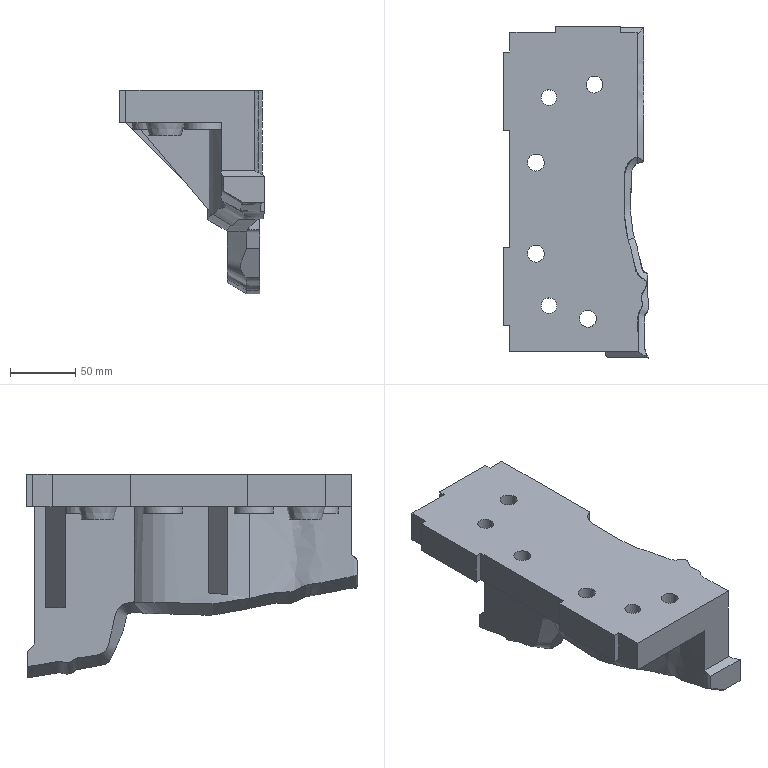Part | NX | features solid 2 | 1 solid | 84 faces | box 111.556 x 254.993 x 156.518 mm | volume 1230678 mm3 | plane 51 | spline 18 | cylinder 13 | cone 2 | commonest cylinder face diameters 13 x6 30 x3 12 x2 32 x2